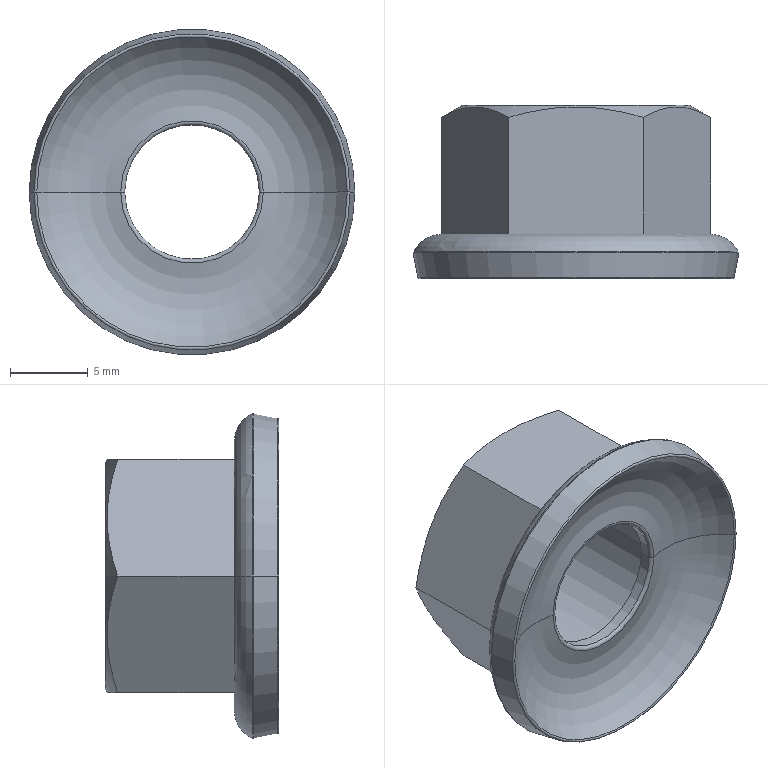Part | STEP file | KOPRESS_M10 | 1 solid | 32 faces | box 20.951 x 11.146 x 20.951 mm | volume 1322 mm3 | plane 14 | torus 10 | cylinder 4 | cone 4 | commonest cylinder face diameters 8.66 x2 10 x2